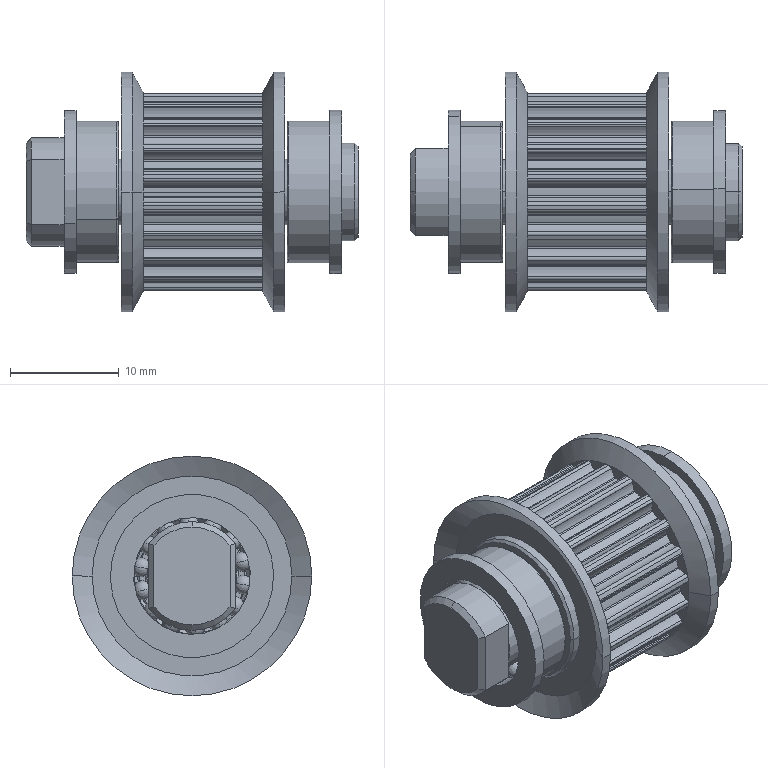Part | SolidWorks | 37 solids | 900 faces | box 30.5 x 22 x 22 mm | volume 4805 mm3 | sphere 304 | cylinder 282 | torus 184 | plane 101 | cone 25 | spline 4 | commonest cylinder face diameters 0.56 x54 0.3 x44 3.95 x42 4 x26 16.12 x21 18.34 x20